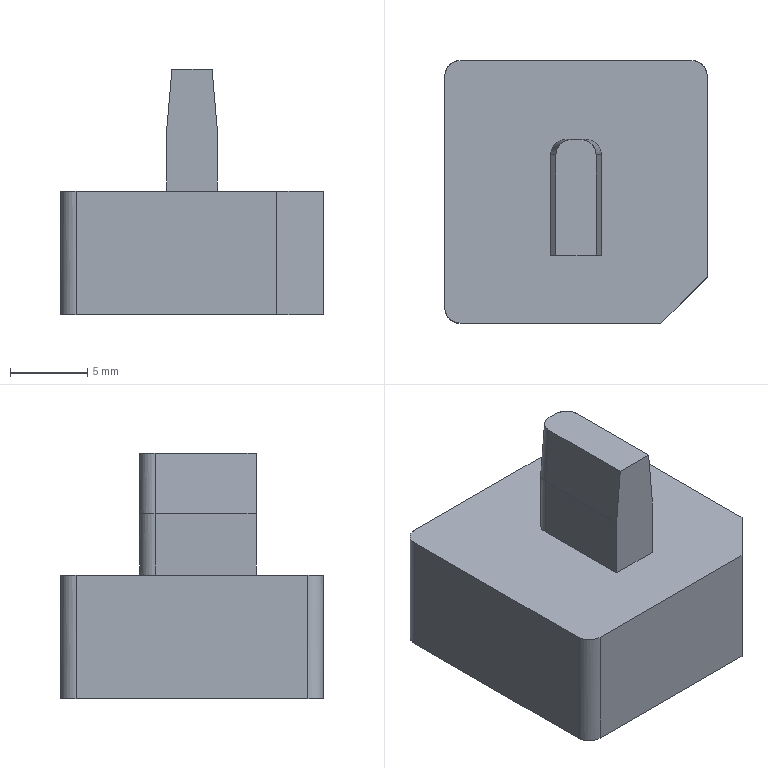NC program | PowerMill | posted with a generic post | part box 17 x 17 x 15.883 mm
Lines 37206 to 37483 of 37483:
N37303 M6
N37304 S15000 M03
N37305 G00 G90 X0.0 Y0.0
N37306 G43 Z10.304 H13
N37307
N37308 G05 P10000 R8
N37309 X-6.0074 Y-7.8023
N37310 Z-8.03
N37311 G01 Z-8.13
N37312 X-6.1108 Y-7.7823 F1000.0
N37313 X-6.1967 Y-7.7432
N37314 X-6.2651 Y-7.6848
N37315 X-6.3149 Y-7.6092
N37316 X-6.3448 Y-7.5183
N37317 X-6.3547 Y-7.412
N37318 X-6.3452 Y-7.3126
N37319 X-6.3165 Y-7.2251
N37320 X-6.2688 Y-7.1497
N37321 X-6.2002 Y-7.0877
N37322 X-6.1177 Y-7.0505
N37323 X-6.0211 Y-7.0382
N37324 X-5.9407 Y-7.0505
N37325 X-5.8584 Y-7.0875
N37326 X-5.7975 Y-7.1411
N37327 X-5.7487 Y-7.1917
N37328 X-5.7281 Y-7.2224
N37329 X-5.6294 Y-7.4607
N37330 X-5.5636 Y-7.5685
N37331 X-5.4827 Y-7.6634
N37332 X-5.3799 Y-7.7481
N37333 X-5.269 Y-7.8035
N37334 X-5.15 Y-7.8297
N37335 Y-7.0372
N37336 G00 Z-4.8788
N37337 G01 X-5.7743 Y-5.7374 F10000.0
N37338 G00 Z-8.03
N37339 G01 Z-8.13 F600.0
N37340 X-5.7339 Y-5.7762 F1000.0
N37341 X-5.6882 Y-5.8426
N37342 X-5.6372 Y-5.9367
N37343 X-5.5925 Y-6.0347
N37344 X-5.5657 Y-6.113
N37345 X-5.5568 Y-6.1716
N37346 X-5.5699 Y-6.272
N37347 X-5.6092 Y-6.3588
N37348 X-5.6747 Y-6.4321
N37349 X-5.7544 Y-6.4844
N37350 X-5.8461 Y-6.5158
N37351 X-5.9498 Y-6.5262
N37352 X-6.0589 Y-6.515
N37353 X-6.1545 Y-6.4815
N37354 X-6.2368 Y-6.4257
N37355 X-6.3023 Y-6.3482
N37356 X-6.3416 Y-6.2559
N37357 X-6.3547 Y-6.1487
N37358 X-6.343 Y-6.043
N37359 X-6.3076 Y-5.9527
N37360 X-6.2488 Y-5.8776
N37361 X-6.1664 Y-5.8178
N37362 X-6.0575 Y-5.7731
N37363 X-5.9267 Y-5.7463
N37364 X-5.7743 Y-5.7374
N37365 X-5.6071 Y-5.7464
N37366 X-5.4639 Y-5.7735
N37367 X-5.3447 Y-5.8187
N37368 X-5.2507 Y-5.8806
N37369 X-5.1836 Y-5.9593
N37370 X-5.1433 Y-6.0547
N37371 X-5.1299 Y-6.167
N37372 X-5.1386 Y-6.2551
N37373 X-5.1648 Y-6.3317
N37374 X-5.2085 Y-6.3969
N37375 X-5.2677 Y-6.4484
N37376 X-5.3405 Y-6.4842
N37377 X-5.427 Y-6.5043
N37378 G00 Z-4.8788
N37379 G01 X-5.5732 Y-4.805 F10000.0
N37380 G00 Z-8.03
N37381 G01 Z-8.13 F600.0
N37382 Y-5.2648 F1000.0
N37383 G00 Z-4.8788
N37384 G01 X-5.5302 Y-3.2574 F10000.0
N37385 G00 Z-8.03
N37386 G01 Z-8.13 F600.0
N37387 X-5.4136 Y-3.2984 F1000.0
N37388 X-5.3157 Y-3.3566
N37389 X-5.2368 Y-3.432
N37390 X-5.1774 Y-3.525
N37391 X-5.1418 Y-3.6323
N37392 X-5.1299 Y-3.7538
N37393 X-5.1422 Y-3.8925
N37394 X-5.179 Y-4.012
N37395 X-5.2405 Y-4.1122
N37396 X-5.3264 Y-4.1931
N37397 X-5.437 Y-4.2547
N37398 X-5.5919 Y-4.302
N37399 X-5.7588 Y-4.3177
N37400 X-5.9043 Y-4.3067
N37401 X-6.0309 Y-4.2737
N37402 X-6.1386 Y-4.2187
N37403 X-6.2273 Y-4.1416
N37404 X-6.2971 Y-4.0426
N37405 X-6.352 Y-3.9037
N37406 X-6.3703 Y-3.7519
N37407 X-6.3603 Y-3.6392
N37408 X-6.3302 Y-3.5387
N37409 X-6.2802 Y-3.4503
N37410 X-6.2113 Y-3.3763
N37411 X-6.1246 Y-3.3187
N37412 X-6.0202 Y-3.2775
N37413 G00 Z-4.8788
N37414 G01 X-5.9296 Y-2.7568 F10000.0
N37415 G00 Z-8.03
N37416 G01 Z-8.13 F600.0
N37417 X-6.0418 Y-2.7373 F1000.0
N37418 X-6.1545 Y-2.6974
N37419 X-6.2421 Y-2.6415
N37420 X-6.3047 Y-2.5697
N37421 X-6.3422 Y-2.4818
N37422 X-6.3547 Y-2.378
N37423 X-6.3422 Y-2.2743
N37424 X-6.3047 Y-2.1864
N37425 X-6.2421 Y-2.1146
N37426 X-6.1545 Y-2.0587
N37427 X-6.0418 Y-2.0188
N37428 X-5.9041 Y-1.9948
N37429 X-5.7414 Y-1.9868
N37430 X-5.5578 Y-1.9977
N37431 X-5.4064 Y-2.0302
N37432 X-5.2872 Y-2.0845
N37433 X-5.2003 Y-2.1605
N37434 X-5.1612 Y-2.2229
N37435 X-5.1377 Y-2.2954
N37436 X-5.1299 Y-2.378
N37437 X-5.1424 Y-2.4818
N37438 X-5.1798 Y-2.5697
N37439 X-5.2422 Y-2.6415
N37440 X-5.3296 Y-2.6974
N37441 X-5.4419 Y-2.7373
N37442 X-5.5792 Y-2.7613
N37443 X-5.7414 Y-2.7693
N37444 X-5.9041 Y-2.7613
N37445 X-5.9296 Y-2.7568
N37446 G00 Z-4.8788
N37447 G01 X-6.1938 Y-1.1568 F10000.0
N37448 G00 Z-8.03
N37449 G01 Z-8.13 F600.0
N37450 X-6.3492 Y-0.931 F1000.0
N37451 X-5.15
N37452 G00 Z-4.8788
N37453 G01 X-5.5732 Y0.2363 F10000.0
N37454 G00 Z-8.03
N37455 G01 Z-8.13 F600.0
N37456 Y-0.2235 F1000.0
N37457 G00 Z-4.8788
N37458 G01 X-5.4599 Y0.7098 F10000.0
N37459 G00 Z-8.03
N37460 G01 Z-8.13 F600.0
N37461 X-5.3615 Y0.7325 F1000.0
N37462 X-5.2795 Y0.7736
N37463 X-5.214 Y0.8332
N37464 X-5.1678 Y0.9073
N37465 X-5.14 Y0.9953
N37466 X-5.1308 Y1.0974
N37467 X-5.1454 Y1.2065
N37468 X-5.1893 Y1.3046
N37469 X-5.2624 Y1.3917
N37470 X-5.3515 Y1.4572
N37471 X-5.4493 Y1.4953
N37472 X-5.5558 Y1.506
N37473 X-5.6809 Y1.4891
N37474 X-5.7789 Y1.4465
N37475 X-5.8498 Y1.3781
N37476 X-5.8937 Y1.284
N37477 X-5.9105 Y1.1641
N37478 X-5.8959 Y1.0656
N37479 X-5.8483 Y0.9493
N37480 X-5.7823 Y0.8394
N37481 X-5.7048 Y0.7473
N37482 X-6.3337 Y0.8506
N37483 Y1.4438
N37484 G00 Z-4.8788
N37485 G01 X-5.5732 Y2.4311 F10000.0
N37486 G00 Z-8.03
N37487 G01 Z-8.13 F600.0
N37488 Y1.9713 F1000.0
N37489 G00 Z-4.8788
N37490 G01 X-5.6194 Y2.9106 F10000.0
N37491 G00 Z-8.03
N37492 G01 Z-8.13 F600.0
N37493 X-5.7414 Y2.9046 F1000.0
N37494 X-5.9041 Y2.9126
N37495 X-6.0418 Y2.9365
N37496 X-6.1545 Y2.9765
N37497 X-6.2421 Y3.0324
N37498 X-6.3047 Y3.1042
N37499 X-6.3422 Y3.192
N37500 X-6.3547 Y3.2958
N37501 X-6.3422 Y3.3996
N37502 X-6.3047 Y3.4874
N37503 X-6.2421 Y3.5593
N37504 X-6.1545 Y3.6152
N37505 X-6.0418 Y3.6551
N37506 X-5.9041 Y3.6791
N37507 X-5.7414 Y3.687
N37508 X-5.5578 Y3.6762
N37509 X-5.4064 Y3.6436
N37510 X-5.2872 Y3.5894
N37511 X-5.2003 Y3.5134
N37512 X-5.1612 Y3.451
N37513 X-5.1377 Y3.3785
N37514 X-5.1299 Y3.2958
N37515 X-5.1424 Y3.192
N37516 X-5.1798 Y3.1042
N37517 X-5.2422 Y3.0324
N37518 X-5.3296 Y2.9765
N37519 X-5.4419 Y2.9365
N37520 X-5.5792 Y2.9126
N37521 X-5.6194 Y2.9106
N37522 G00 Z-4.8788
N37523 G01 X-5.2103 Y4.3452 F10000.0
N37524 G00 Z-8.03
N37525 G01 Z-8.13 F600.0
N37526 X-5.3763 F1000.0
N37527 G00 Z-4.8788
N37528 G01 X-5.4957 Y5.0296 F10000.0
N37529 G00 Z-8.03
N37530 G01 Z-8.13 F600.0
N37531 X-5.5792 Y5.0151 F1000.0
N37532 X-5.7414 Y5.0071
N37533 X-5.9041 Y5.0151
N37534 X-6.0418 Y5.039
N37535 X-6.1545 Y5.0789
N37536 X-6.2421 Y5.1348
N37537 X-6.3047 Y5.2067
N37538 X-6.3422 Y5.2945
N37539 X-6.3547 Y5.3983
N37540 X-6.3422 Y5.5021
N37541 X-6.3047 Y5.5899
N37542 X-6.2421 Y5.6618
N37543 X-6.1545 Y5.7176
N37544 X-6.0418 Y5.7576
N37545 X-5.9041 Y5.7815
N37546 X-5.7414 Y5.7895
N37547 X-5.5578 Y5.7786
N37548 X-5.4064 Y5.7461
N37549 X-5.2872 Y5.6918
N37550 X-5.2003 Y5.6158
N37551 X-5.1612 Y5.5535
N37552 X-5.1377 Y5.481
N37553 X-5.1299 Y5.3983
N37554 X-5.1424 Y5.2945
N37555 X-5.1798 Y5.2067
N37556 X-5.2422 Y5.1348
N37557 X-5.3296 Y5.0789
N37558 X-5.4419 Y5.039
N37559 X-5.4957 Y5.0296
N37560 G00 Z-4.8788
N37561 G01 X-6.3337 Y6.3005 F10000.0
N37562 G00 Z-8.03
N37563 G01 Z-8.13 F600.0
N37564 Y7.0766 F1000.0
N37565 X-6.2329 Y7.0384
N37566 X-6.1098 Y6.9751
N37567 X-5.895 Y6.8499
N37568 X-5.6489 Y6.7337
N37569 X-5.4006 Y6.6569
N37570 X-5.15 Y6.6195
N37571 G00 Z10.304
N37572 G05 P0
N37573 (---------------)
N37574 ( END TOOLPATH : 精公刻字01-刻字-TEXT_D4 )
N37575 (---------------)
N37576
N37577 M05
N37578 G53 Z0.0
N37579 M30
%